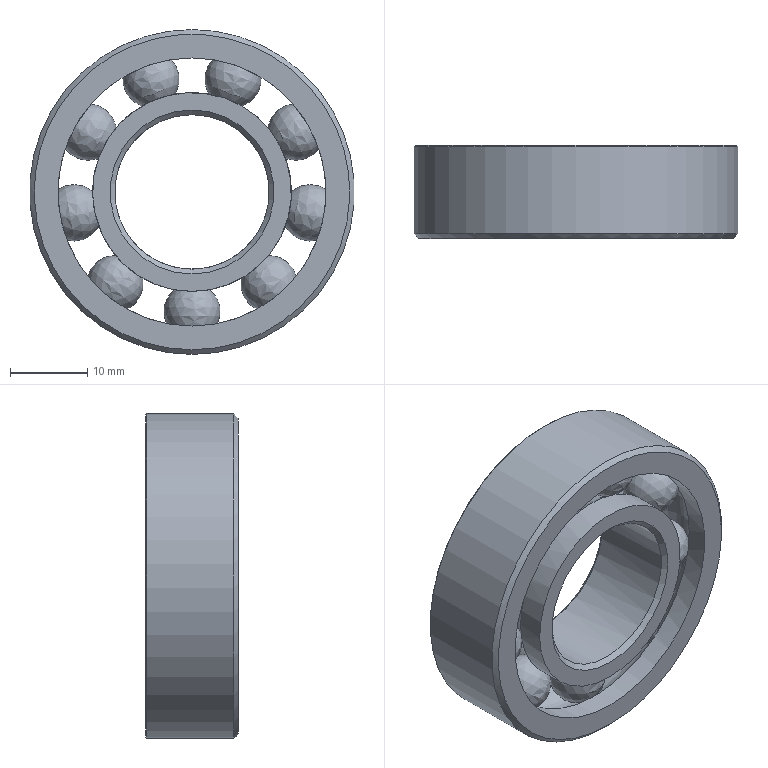Part | STEP file | 冲床-300配套压波_id1062_x_t | 1 solid | 41 faces | box 42 x 12 x 42 mm | volume 8257 mm3 | torus 18 | sphere 9 | cylinder 5 | cone 5 | plane 4 | commonest cylinder face diameters 25.7 x2 20 x1 34.666 x1 42 x1